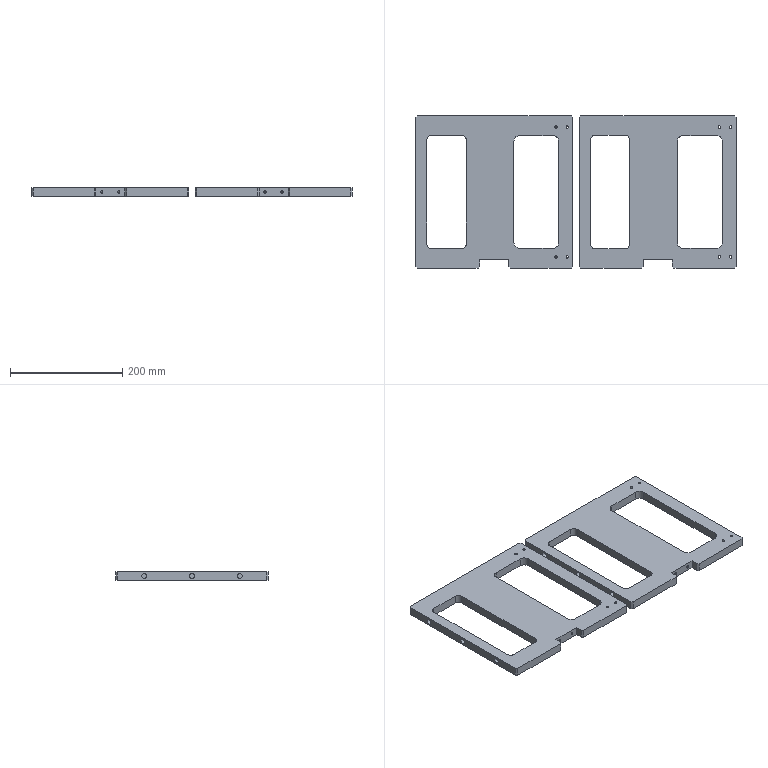CAM job | NX | 3-axis milling, drilling | part box 570 x 271 x 15 mm | stock box 575 x 276 x 15 mm
Tools:
number,name,description,diameter,corner_radius,flute_length,length,flutes
9,D10,平底铣刀-粗,10.0,0.0,35.0,75.0,2
11,D3-J,平底铣刀-精,3.0,0.0,50.0,75.0,2
7,D6-J,平底铣刀-精,6.0,0.0,25.0,75.0,2
2,D6倒角刀,倒角刀,6.0,0.0,3.0,25.0,2
14,ZT4.3,Drilling Tool,4.3,0.0,50.0,75.0,4
Operations:
program,operation,operation_type,tool,method,geometry_group,spindle_rpm,surface_speed,feed_per_tooth,feed_cut,feed_plunge,cut_length_mm,path_length_mm,cut_time_min,machine_time_min
B,C0.3-CONTOURCHAMFER6X45L_COPY,PlanarMilling,D6倒角刀,CLIMBCHAMFER-DEPTH0-STEPG,W-B,7000.0,131.0,0.1071,1500.0,100.0,2226.099,2736.478,1.484,1.535
B,DRILL-CHAMFER_2,Operation,D6倒角刀,METHOD,W-B,8000.0,150.796,0.0625,1000.0,0.0,22.8,426.067,0.0228,0.0631
A,SPOTTING,Operation,D6倒角刀,METHOD,W-A,3000.0,56.549,0.0333,200.0,0.0,20.0,919.606,0.1,0.19
A,DRILLHOLES,Operation,ZT4.3,METHOD,W-A,3000.0,39.584,0.0167,100.0,0.0,124.0,1127.606,1.24,1.34
A,POCKET-ROUGH_1,VolumeBased25DMillingOperation,D10,METHOD,W-A,6000.0,188.0,0.25,4000.0,80.0,31671.846,32108.347,7.918,7.962
A,POCKET-ROUGH_2,VolumeBased25DMillingOperation,D10,METHOD,W-A,6000.0,188.0,0.25,4000.0,80.0,30768.732,31205.232,7.692,7.736
A,PROFILE-ROUGH_2,VolumeBased25DMillingOperation,D10,METHOD,W-A,6000.0,188.0,0.25,4000.0,80.0,71186.583,71622.583,17.797,17.84
A,POCKET-SEMIFIN_1,VolumeBased25DMillingOperation,D6-J,METHOD,W-A,6000.0,113.0,0.0833,1000.0,100.0,2116.431,2583.697,2.116,2.163
A,POCKET-SEMIFIN_2,VolumeBased25DMillingOperation,D6-J,METHOD,W-A,6000.0,113.0,0.0833,1000.0,100.0,2058.338,2525.816,2.058,2.105
A,POCKET-FINISH_1,VolumeBased25DMillingOperation,D6-J,METHOD,W-A,6000.0,113.0,0.0833,1000.0,100.0,1057.816,1525.443,1.058,1.105
A,POCKET-FINISH_2,VolumeBased25DMillingOperation,D6-J,METHOD,W-A,6000.0,113.0,0.0833,1000.0,100.0,1028.769,1496.607,1.029,1.076
A,BOTTOMWALL-HELIXFIN-MID_COPY,VolumeBased25DMillingOperation,D3-J,HELIX-FINISH-DEPTHK-STEPG,W-A,8000.0,50.266,0.0187,300.0,100.0,1421.769,2819.511,4.739,4.879
A,PROFILE-D4-CLEAR,ZLevelMilling,D3-J,METHOD,W-A,6000.0,75.0,0.25,2500.0,80.0,2508.998,3022.847,1.004,1.055
A,CHAMFER_2,SurfaceContour,D6倒角刀,METHOD,W-A,6000.0,113.0,0.125,1200.0,100.0,4419.379,5514.958,3.683,3.792
A,DRILL-CHAMFER_1,Operation,D6倒角刀,METHOD,W-A,5000.0,94.248,0.015,150.0,0.0,45.6,985.651,0.304,0.398
A,PROFILE-SEMIFIN_2,VolumeBased25DMillingOperation,D6-J,METHOD,W-A,6000.0,113.0,0.0833,1000.0,100.0,4566.586,5187.644,4.567,4.629
A,PROFILE-FINISH_2,VolumeBased25DMillingOperation,D6-J,METHOD,W-A,6000.0,113.0,0.0833,1000.0,100.0,2282.893,2753.098,2.283,2.33